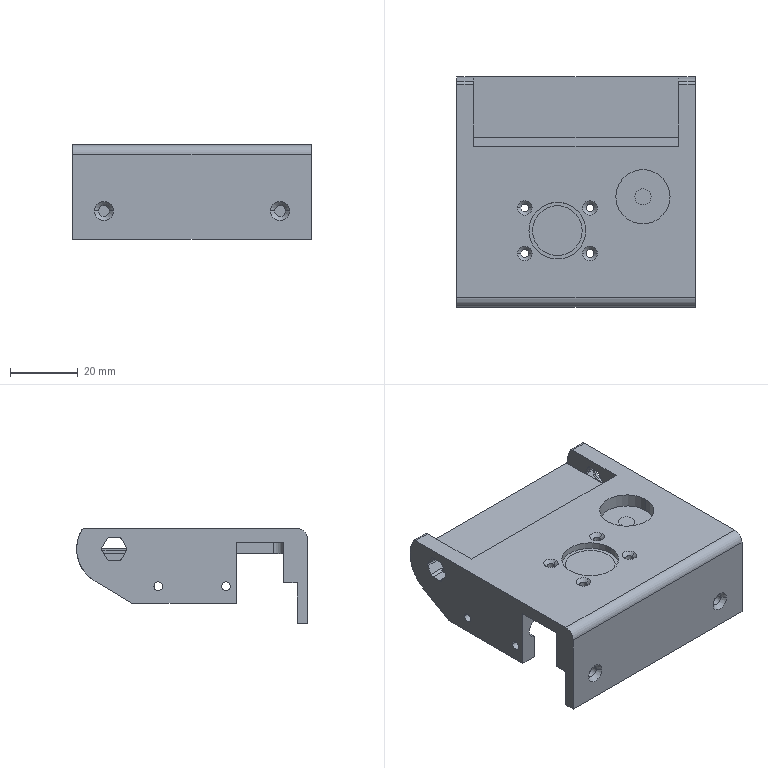NC program | NX | posted with a generic post | part box 70.5 x 68.1 x 28 mm
Lines 4053 to 5120 of 7250:
(ZLEVEL_PROFILE_COPY_COPY_1_COPY_1_COPY_1 , TOOL : D6R0.5)
N8062 T05 M6
N8064 G54
N8066 G17 G0 G90 X55.649 Y-26.288 B0. C0. S9500 M3
N8068 G43 Z30. H5
N8070 Z-5.051
N8072 G94 G1 Z-6.051 F1000.
N8074 X55.011 Y-26.4
N8076 G3 X54.516 Y-26.991 R0.6
N8078 G1 X54.515 Y-38.509 F3000.
N8080 X54.56 Y-38.51 Z-6.077
N8082 X54.601 Z-6.102
N8084 X54.603 Y-35.25
N8086 Y-30.25
N8088 X54.602 Y-26.99
N8090 X54.646 Z-6.128
N8092 X54.688 Y-26.989 Z-6.153
N8094 X54.689 Y-30.25
N8096 Y-35.25
N8098 X54.687 Y-38.511
N8100 X54.732 Z-6.179
N8102 X54.773 Y-38.512 Z-6.204
N8104 X54.775 Y-35.25
N8106 Y-30.25
N8108 X54.774 Y-26.989
N8110 X54.818 Y-26.988 Z-6.23
N8112 X54.86 Z-6.255
N8114 X54.861 Y-30.25
N8116 Y-35.25
N8118 X54.859 Y-38.512
N8120 X54.904 Y-38.513 Z-6.281
N8122 X54.945 Z-6.306
N8124 X54.947 Y-35.25
N8126 Y-30.25
N8128 X54.946 Y-26.987
N8130 X54.99 Z-6.332
N8132 X55.032 Y-26.986 Z-6.357
N8134 X55.033 Y-30.25
N8136 Y-35.25
N8138 X55.031 Y-38.514
N8140 X55.076 Z-6.383
N8142 X55.117 Y-38.515 Z-6.408
N8144 X55.119 Y-35.25
N8146 Y-30.25
N8148 X55.118 Y-26.986
N8150 X55.162 Y-26.985 Z-6.434
N8152 X55.204 Z-6.459
N8154 X55.205 Y-30.25
N8156 Y-35.25
N8158 X55.203 Y-38.515
N8160 X55.248 Y-38.516 Z-6.485
N8162 X55.289 Z-6.511
N8164 X55.29 Y-35.25
N8166 Y-30.25
N8168 Y-26.984
N8170 X55.333 Z-6.536
N8172 X55.376 Y-26.983 Z-6.562
N8174 Y-30.25
N8176 Y-35.25
N8178 X55.375 Y-38.517
N8180 X55.419 Z-6.587
N8182 X55.461 Y-38.518 Z-6.613
N8184 X55.462 Y-35.25
N8186 Y-30.25
N8188 Y-26.983
N8190 X55.505 Y-26.982 Z-6.638
N8192 X55.548 Z-6.664
N8194 Y-30.25
N8196 Y-35.25
N8198 X55.547 Y-38.518
N8200 X55.591 Y-38.519 Z-6.689
N8202 X55.633 Z-6.715
N8204 X55.634 Y-35.25
N8206 Y-30.25
N8208 Y-26.981
N8210 X55.677 Z-6.74
N8212 X55.72 Y-26.98 Z-6.766
N8214 Y-30.25
N8216 Y-35.25
N8218 X55.719 Y-38.52
N8220 X55.763 Z-6.791
N8222 X55.805 Y-38.521 Z-6.817
N8224 X55.806 Y-35.25
N8226 Y-30.25
N8228 Y-26.98
N8230 X55.849 Y-26.979 Z-6.842
N8232 X55.892 Z-6.868
N8234 Y-30.25
N8236 Y-35.25
N8238 X55.891 Y-38.521
N8240 X55.935 Y-38.522 Z-6.893
N8242 X55.977 Z-6.919
N8244 X55.978 Y-35.25
N8246 Y-30.25
N8248 Y-26.978
N8250 X56.021 Z-6.944
N8252 X56.064 Y-26.977 Z-6.97
N8254 Y-30.25
N8256 Y-35.25
N8258 X56.063 Y-38.523
N8260 X56.107 Z-6.995
N8262 X56.149 Z-7.021
N8264 X56.15 Y-35.25
N8266 Y-30.25
N8268 Y-26.977
N8270 X56.193 Z-7.047
N8272 X56.236 Y-26.976 Z-7.072
N8274 Y-30.25
N8276 Y-35.25
N8278 X56.235 Y-38.524
N8280 X56.279 Z-7.098
N8282 X56.321 Y-38.525 Z-7.123
N8284 X56.322 Y-35.25
N8286 Y-30.25
N8288 Y-26.976
N8290 X56.365 Y-26.975 Z-7.149
N8292 X56.408 Z-7.174
N8294 Y-30.25
N8296 Y-35.25
N8298 X56.407 Y-38.525
N8300 X56.451 Y-38.526 Z-7.2
N8302 X56.493 Z-7.225
N8304 X56.494 Y-35.25
N8306 Y-30.25
N8308 Y-26.974
N8310 X56.537 Z-7.251
N8312 X56.58 Z-7.276
N8314 Y-30.25
N8316 Y-35.25
N8318 X56.579 Y-38.527
N8320 X56.623 Z-7.302
N8322 X56.665 Z-7.327
N8324 X56.666 Y-35.25
N8326 Y-30.25
N8328 Y-26.973
N8330 X56.709 Z-7.353
N8332 X56.752 Y-26.972 Z-7.378
N8334 Y-30.25
N8336 Y-35.25
N8338 X56.751 Y-38.528
N8340 X56.795 Z-7.404
N8342 X56.837 Z-7.429
N8344 X56.838 Y-35.25
N8346 Y-30.25
N8348 Y-26.972
N8350 X56.881 Y-26.971 Z-7.455
N8352 X56.924 Z-7.48
N8354 Y-30.25
N8356 Y-35.25
N8358 X56.923 Y-38.529
N8360 X56.967 Z-7.506
N8362 X57.009 Y-38.53 Z-7.532
N8364 X57.01 Y-35.25
N8366 Y-30.25
N8368 Y-26.971
N8370 X57.053 Y-26.97 Z-7.557
N8372 X57.096 Z-7.583
N8374 Y-30.25
N8376 Y-35.25
N8378 X57.095 Y-38.53
N8380 X57.139 Y-38.531 Z-7.608
N8382 X57.181 Z-7.634
N8384 X57.182 Y-35.25
N8386 Y-30.25
N8388 Y-26.969
N8390 X57.225 Z-7.659
N8392 X57.268 Z-7.685
N8394 Y-30.25
N8396 Y-35.25
N8398 X57.267 Y-38.532
N8400 X57.311 Z-7.71
N8402 X57.353 Z-7.736
N8404 X57.354 Y-35.25
N8406 Y-30.25
N8408 Y-26.968
N8410 X57.397 Z-7.761
N8412 X57.44 Z-7.787
N8414 Y-30.25
N8416 Y-35.25
N8418 X57.439 Y-38.533
N8420 X57.483 Z-7.812
N8422 X57.525 Z-7.838
N8424 X57.526 Y-35.25
N8426 Y-30.25
N8428 Y-26.967
N8430 X57.569 Z-7.863
N8432 X57.612 Y-26.966 Z-7.889
N8434 Y-30.25
N8436 Y-35.25
N8438 X57.611 Y-38.534
N8440 X57.655 Z-7.914
N8442 X57.697 Z-7.94
N8444 X57.698 Y-35.25
N8446 Y-30.25
N8448 Y-26.966
N8450 X57.741 Z-7.965
N8452 X57.784 Y-26.965 Z-7.991
N8454 Y-30.25
N8456 Y-35.25
N8458 X57.783 Y-38.535
N8460 X57.827 Z-8.016
N8462 X57.869 Z-8.042
N8464 X57.87 Y-35.25
N8466 Y-30.25
N8468 Y-26.965
N8470 X57.913 Z-8.068
N8472 X57.956 Z-8.093
N8474 Y-30.25
N8476 Y-35.25
N8478 X57.955 Y-38.536
N8480 X57.999 Z-8.119
N8482 X58.041 Z-8.144
N8484 X58.042 Y-35.25
N8486 Y-30.25
N8488 Y-26.964
N8490 X58.085 Z-8.17
N8492 X58.128 Z-8.195
N8494 Y-30.25
N8496 Y-35.25
N8498 X58.127 Y-38.536
N8500 X58.171 Y-38.537 Z-8.221
N8502 X58.213 Z-8.246
N8504 X58.214 Y-35.25
N8506 Y-30.25
N8508 Y-26.964
N8510 X58.257 Y-26.963 Z-8.272
N8512 X58.3 Z-8.297
N8514 Y-30.25
N8516 Y-35.25
N8518 X58.299 Y-38.537
N8520 X58.343 Z-8.323
N8522 X58.385 Y-38.538 Z-8.348
N8524 X58.386 Y-35.25
N8526 Y-30.25
N8528 Y-26.963
N8530 X58.429 Z-8.374
N8532 X58.472 Y-26.962 Z-8.399
N8534 Y-30.25
N8536 Y-35.25
N8538 X58.471 Y-38.538
N8540 X58.515 Z-8.425
N8542 X58.557 Z-8.45
N8544 X58.558 Y-35.25
N8546 Y-30.25
N8548 Y-26.962
N8550 X58.601 Z-8.476
N8552 X58.644 Z-8.501
N8554 Y-30.25
N8556 Y-35.25
N8558 X58.643 Y-38.539
N8560 X58.687 Z-8.527
N8562 X58.729 Z-8.553
N8564 X58.73 Y-35.25
N8566 Y-30.25
N8568 Y-26.961
N8570 X58.773 Z-8.578
N8572 X58.816 Z-8.604
N8574 Y-30.25
N8576 Y-35.25
N8578 X58.815 Y-38.54
N8580 X58.859 Z-8.629
N8582 X58.901 Z-8.655
N8584 X58.902 Y-35.25
N8586 Y-30.25
N8588 Y-26.961
N8590 X58.945 Y-26.96 Z-8.68
N8592 X58.988 Z-8.706
N8594 Y-30.25
N8596 Y-35.25
N8598 X58.987 Y-38.54
N8600 X59.031 Y-38.541 Z-8.731
N8602 X59.073 Z-8.757
N8604 X59.074 Y-35.25
N8606 Y-30.25
N8608 Y-26.96
N8610 X59.117 Z-8.782
N8612 X59.16 Z-8.808
N8614 Y-30.25
N8616 Y-35.25
N8618 X59.159 Y-38.541
N8620 X59.203 Z-8.833
N8622 X59.245 Z-8.859
N8624 X59.246 Y-35.25
N8626 Y-30.25
N8628 X59.245 Y-26.959
N8630 X59.289 Z-8.884
N8632 X59.331 Z-8.91
N8634 X59.332 Y-30.25
N8636 Y-35.25
N8638 X59.331 Y-38.542
N8640 X59.375 Z-8.935
N8642 X59.417 Z-8.961
N8644 X59.418 Y-35.25
N8646 Y-30.25
N8648 X59.417 Y-26.959
N8650 X59.461 Z-8.986
N8652 X59.503 Z-9.012
N8654 X59.504 Y-30.25
N8656 Y-35.25
N8658 X59.503 Y-38.542
N8660 X59.547 Z-9.038
N8662 X59.589 Y-38.543 Z-9.063
N8664 X59.59 Y-35.25
N8666 Y-30.25
N8668 X59.589 Y-26.958
N8670 X59.633 Z-9.089
N8672 X59.675 Z-9.114
N8674 X59.676 Y-30.25
N8676 Y-35.25
N8678 X59.675 Y-38.543
N8680 X59.719 Z-9.14
N8682 X59.761 Z-9.165
N8684 X59.762 Y-35.25
N8686 Y-30.25
N8688 X59.761 Y-26.958
N8690 X59.805 Z-9.191
N8692 X59.847 Z-9.216
N8694 X59.848 Y-30.25
N8696 Y-35.25
N8698 X59.847 Y-38.543
N8700 X59.891 Z-9.242
N8702 X59.933 Z-9.267
N8704 X59.934 Y-35.25
N8706 Y-30.25
N8708 X59.933 Y-26.958
N8710 X59.977 Z-9.293
N8712 X60.019 Z-9.318
N8714 X60.02 Y-30.25
N8716 Y-35.25
N8718 X60.019 Y-38.544
N8720 X60.063 Z-9.344
N8722 X60.105 Z-9.369
N8724 X60.106 Y-35.25
N8726 Y-30.25
N8728 X60.105 Y-26.957
N8730 X60.149 Z-9.395
N8732 X60.191 Z-9.42
N8734 X60.192 Y-30.25
N8736 Y-35.25
N8738 X60.191 Y-38.544
N8740 X60.235 Z-9.446
N8742 X60.277 Z-9.471
N8744 X60.278 Y-35.25
N8746 Y-30.25
N8748 X60.277 Y-26.957
N8750 X60.321 Z-9.497
N8752 X60.363 Z-9.522
N8754 X60.364 Y-30.25
N8756 Y-35.25
N8758 X60.363 Y-38.544
N8760 X60.407 Y-38.545 Z-9.548
N8762 X60.449 Z-9.574
N8764 X60.45 Y-35.25
N8766 Y-30.25
N8768 X60.449 Y-26.957
N8770 X60.493 Z-9.599
N8772 X60.535 Z-9.625
N8774 X60.536 Y-30.25
N8776 Y-35.25
N8778 X60.535 Y-38.545
N8780 X60.579 Z-9.65
N8782 X60.621 Z-9.676
N8784 X60.622 Y-35.25
N8786 Y-30.25
N8788 X60.621 Y-26.956
N8790 X60.665 Z-9.701
N8792 X60.707 Z-9.727
N8794 X60.708 Y-30.25
N8796 Y-35.25
N8798 X60.707 Y-38.545
N8800 X60.751 Y-38.546 Z-9.752
N8802 X60.793 Z-9.778
N8804 X60.794 Y-35.25
N8806 Y-30.25
N8808 X60.793 Y-26.956
N8810 X60.837 Z-9.803
N8812 X60.879 Z-9.829
N8814 X60.88 Y-30.25
N8816 Y-35.25
N8818 X60.879 Y-38.546
N8820 X60.923 Z-9.854
N8822 X60.965 Z-9.88
N8824 X60.966 Y-35.25
N8826 Y-30.25
N8828 X60.965 Y-26.956
N8830 X61.009 Z-9.905
N8832 X61.051 Z-9.931
N8834 X61.052 Y-30.25
N8836 Y-35.25
N8838 X61.051 Y-38.546
N8840 X61.095 Z-9.956
N8842 X61.137 Z-9.982
N8844 X61.138 Y-35.25
N8846 Y-30.25
N8848 X61.137 Y-26.956
N8850 X61.181 Z-10.007
N8852 X61.223 Z-10.033
N8854 X61.224 Y-30.25
N8856 Y-35.25
N8858 X61.223 Y-38.546
N8860 X61.267 Z-10.059
N8862 X61.309 Z-10.084
N8864 X61.31 Y-35.25
N8866 Y-30.25
N8868 X61.309 Y-26.956
N8870 X61.353 Z-10.11
N8872 X61.395 Z-10.135
N8874 X61.396 Y-30.25
N8876 Y-35.25
N8878 X61.395 Y-38.547
N8880 X61.439 Z-10.161
N8882 X61.481 Z-10.186
N8884 X61.482 Y-35.25
N8886 Y-30.25
N8888 X61.481 Y-26.956
N8890 X61.525 Z-10.212
N8892 X61.567 Z-10.237
N8894 X61.568 Y-30.25
N8896 Y-35.25
N8898 X61.567 Y-38.547
N8900 X61.611 Z-10.263
N8902 X61.653 Z-10.288
N8904 X61.654 Y-35.25
N8906 Y-30.25
N8908 X61.653 Y-26.956
N8910 X61.697 Z-10.314
N8912 X61.739 Z-10.339
N8914 X61.74 Y-30.25
N8916 Y-35.25
N8918 X61.739 Y-38.547
N8920 X61.782 Z-10.365
N8922 X61.825 Z-10.39
N8924 X61.826 Y-35.25
N8926 Y-30.25
N8928 X61.825 Y-26.956
N8930 X61.869 Z-10.416
N8932 X61.911 Z-10.441
N8934 X61.912 Y-30.25
N8936 Y-35.25
N8938 X61.911 Y-38.547
N8940 X61.954 Z-10.467
N8942 X61.997 Z-10.492
N8944 X61.998 Y-35.25
N8946 Y-30.25
N8948 X61.997 Y-26.956
N8950 X62.041 Z-10.518
N8952 X62.083 Z-10.543
N8954 X62.084 Y-30.25
N8956 Y-35.25
N8958 X62.083 Y-38.548
N8960 X62.126 Z-10.569
N8962 X62.169 Z-10.595
N8964 Y-35.25
N8966 Y-30.25
N8968 Y-26.956
N8970 X62.212 Z-10.62
N8972 X62.255 Z-10.646
N8974 Y-30.25
N8976 Y-35.25
N8978 Y-38.548
N8980 X62.298 Z-10.671
N8982 X62.34 Z-10.697
N8984 X62.341 Y-35.25
N8986 Y-30.25
N8988 Y-26.956
N8990 X62.384 Z-10.722
N8992 X62.427 Z-10.748
N8994 Y-30.25
N8996 Y-35.25
N8998 X62.426 Y-38.548
N9000 X62.47 Z-10.773
N9002 X62.512 Z-10.799
N9004 X62.513 Y-35.25
N9006 Y-30.25
N9008 Y-26.956
N9010 X62.556 Z-10.824
N9012 X62.599 Z-10.85
N9014 X62.598 Y-30.007
N9016 X62.599 Y-30.25
N9018 Y-35.25
N9020 X62.598 Y-38.275
N9022 Y-38.548
N9024 X62.642 Z-10.875
N9026 X62.684 Z-10.901
N9028 X62.682 Y-37.931
N9030 X62.685 Y-35.25
N9032 Y-30.25
N9034 X62.684 Y-30.007
N9036 X62.685 Y-26.956
N9038 X62.728 Z-10.926
N9040 X62.771 Y-26.957 Z-10.952
N9042 X62.769 Y-30.007
N9044 X62.771 Y-30.25
N9046 Y-35.25
N9048 X62.768 Y-37.931
N9050 X62.77 Y-38.548
N9052 X62.814 Z-10.977
N9054 X62.856 Z-11.003
N9056 X62.853 Y-37.931
N9058 X62.857 Y-35.25
N9060 Y-30.25
N9062 X62.855 Y-30.007
N9064 X62.857 Y-26.957
N9066 X62.9 Z-11.028
N9068 X62.943 Z-11.054
N9070 X62.939 Y-29.663
N9072 X62.943 Y-30.25
N9074 Y-35.25
N9076 X62.941 Y-38.275
N9078 X62.942 Y-38.548
N9080 X62.986 Z-11.08
N9082 X63.028 Z-11.105
N9084 X63.025 Y-37.931
N9086 X63.029 Y-35.25
N9088 Y-30.25
N9090 X63.025 Y-29.663
N9092 X63.029 Y-26.957
N9094 X63.072 Z-11.131
N9096 X63.115 Z-11.156
N9098 X63.111 Y-29.663
N9100 X63.115 Y-30.25
N9102 Y-35.25
N9104 X63.111 Y-37.931
N9106 X63.114 Y-38.548
N9108 X63.158 Z-11.182
N9110 X63.2 Z-11.207
N9112 X63.197 Y-37.931
N9114 X63.201 Y-35.25
N9116 Y-30.25
N9118 X63.196 Y-29.663
N9120 X63.201 Y-26.957
N9122 X63.244 Z-11.233
N9124 X63.287 Z-11.258
N9126 X63.282 Y-29.663
N9128 X63.287 Y-30.25
N9130 Y-35.25
N9132 X63.285 Y-38.549
N9134 X63.33 Z-11.284
N9136 X63.371 Z-11.309
N9138 X63.373 Y-35.25
N9140 Y-30.25
N9142 X63.368 Y-29.663
N9144 X63.373 Y-26.957
N9146 X63.416 Z-11.335
N9148 X63.459 Y-26.958 Z-11.36
N9150 X63.454 Y-29.663
N9152 X63.459 Y-30.25
N9154 Y-35.25
N9156 X63.457 Y-38.549
N9158 X63.501 Z-11.386
N9160 X63.543 Z-11.411
N9162 X63.545 Y-35.25
N9164 Y-30.25
N9166 X63.539 Y-29.663
N9168 X63.545 Y-26.958
N9170 X63.588 Z-11.437
N9172 X63.63 Z-11.462
N9174 X63.625 Y-29.663
N9176 X63.631 Y-30.25
N9178 Y-35.25
N9180 X63.629 Y-38.549
N9182 X63.673 Z-11.488
N9184 X63.715 Z-11.513
N9186 X63.716 Y-35.519
N9188 X63.717 Y-35.25
N9190 Y-30.25
N9192 X63.711 Y-29.663
N9194 X63.716 Y-26.958
N9196 X63.76 Z-11.539
N9198 X63.802 Z-11.564
N9200 X63.797 Y-29.663
N9202 X63.803 Y-30.25
N9204 Y-35.25
N9206 X63.8 Y-35.864
N9208 X63.801 Y-38.549
N9210 X63.845 Z-11.59
N9212 X63.887 Z-11.616
N9214 X63.885 Y-35.864
N9216 X63.889 Y-35.25
N9218 Y-30.25
N9220 X63.883 Y-29.663
N9222 X63.888 Y-26.958
N9224 X63.932 Y-26.959 Z-11.641
N9226 X63.974 Z-11.667
N9228 X63.971 Y-30.007
N9230 X63.975 Y-30.25
N9232 Y-35.25
N9234 X63.972 Y-38.549
N9236 X64.016 Z-11.692
N9238 X64.057 Z-11.718
N9240 X64.061 Y-35.25
N9242 Y-30.25
N9244 X64.051 Y-29.663
N9246 X64.059 Y-26.959
N9248 X64.102 Z-11.743
N9250 X64.144 Z-11.769
N9252 X64.135 Y-29.663
N9254 X64.147 Y-30.25
N9256 Y-35.25
N9258 X64.142 Y-38.549
N9260 X64.186 Z-11.794
N9262 X64.227 Z-11.82
N9264 X64.223 Y-38.275
N9266 X64.233 Y-35.25
N9268 Y-30.25
N9270 X64.219 Y-29.663
N9272 X64.23 Y-26.96
N9274 X64.273 Z-11.845
N9276 X64.315 Z-11.871
N9278 X64.303 Y-29.663
N9280 X64.319 Y-30.25
N9282 Y-35.25
N9284 X64.301 Y-37.931
N9286 X64.312 Y-38.549
N9288 X64.356 Z-11.896
N9290 X64.397 Z-11.922
N9292 X64.385 Y-37.931
N9294 X64.405 Y-35.25
N9296 Y-30.25
N9298 X64.387 Y-29.663
N9300 X64.401 Y-26.96
N9302 X64.444 Z-11.947
N9304 X64.486 Y-26.961 Z-11.973
N9306 X64.482 Y-30.007
N9308 X64.491 Y-30.25
N9310 Y-35.25
N9312 X64.469 Y-37.931
N9314 X64.482 Y-38.549
N9316 X64.527 Z-11.998
N9318 X64.567 Z-12.024
N9320 G2 X64.577 Y-35.25 R56.425
N9322 G1 Y-30.25
N9324 X64.554 Y-29.663
N9326 X64.572 Y-26.961
N9328 X64.615 Z-12.049
N9330 X64.657 Z-12.075
N9332 X64.639 Y-29.663
N9334 X64.663 Y-30.25
N9336 Y-35.25
N9338 G3 X64.653 Y-38.549 R51.896
N9340 G1 X64.697 Z-12.101
N9342 X64.738 Z-12.126
N9344 G2 X64.749 Y-35.25 R48.139
N9346 G1 Y-30.25
N9348 X64.724 Y-29.663
N9350 X64.742 Y-26.962
N9352 X64.786 Z-12.152
N9354 X64.828 Z-12.177
N9356 X64.809 Y-29.663
N9358 X64.835 Y-30.25
N9360 Y-35.25
N9362 G3 X64.823 Y-38.549 R44.89
N9364 G1 X64.868 Y-38.55 Z-12.203
N9366 X64.908 Z-12.228
N9368 G2 X64.921 Y-35.25 R42.052
N9370 G1 Y-30.25
N9372 X64.894 Y-29.663
N9374 X64.913 Y-26.962
N9376 X64.957 Z-12.254
N9378 X64.999 Y-26.963 Z-12.279
N9380 X64.996 Y-27.251
N9382 X64.98 Y-29.663
N9384 X65.007 Y-30.25
N9386 Y-35.25
N9388 G3 X64.993 Y-38.55 R39.225
N9390 G1 X65.038 Z-12.305
N9392 X65.078 Z-12.33
N9394 G2 X65.093 Y-35.25 R37.273
N9396 G1 Y-30.25
N9398 G2 X65.084 Y-26.963 R41.614
N9400 G1 X65.128 Z-12.356
N9402 X65.169 Z-12.381
N9404 G3 X65.179 Y-30.25 R39.32
N9406 G1 Y-35.25
N9408 G3 X65.164 Y-38.55 R35.506
N9410 G1 X65.208 Z-12.407
N9412 X65.249 Z-12.432
N9414 G2 X65.265 Y-35.25 R33.187
N9416 G1 Y-30.25
N9418 G2 X65.255 Y-26.964 R37.265
N9420 G1 X65.299 Z-12.458
N9422 X65.337 Z-12.483
N9424 G3 X65.351 Y-30.25 R34.656
N9426 G1 Y-35.25
N9428 G3 X65.331 Y-38.55 R31.308
N9430 G1 X65.379 Z-12.509
N9432 X65.412 Z-12.534
N9434 G2 X65.437 Y-35.25 R29.3
N9436 G1 Y-30.25
N9438 G2 X65.418 Y-26.965 R31.712
N9440 G1 X65.466 Z-12.56
N9442 X65.5 Z-12.586
N9444 G3 X65.523 Y-30.25 R29.549
N9446 G1 Y-35.25
N9448 G3 X65.493 Y-38.55 R27.132
N9450 G1 X65.54 Z-12.612
N9452 X65.576 Z-12.638
N9454 G2 X65.608 Y-35.25 R25.738
N9456 G1 Y-30.25
N9458 G2 X65.582 Y-26.966 R28.254
N9460 G1 X65.626 Z-12.665
N9462 X65.664 Z-12.691
N9464 G3 X65.692 Y-30.25 R27.78
N9466 G1 Y-35.25
N9468 G3 X65.658 Y-38.55 R24.917
N9470 G1 X65.701 Z-12.718
N9472 X65.739 Z-12.744
N9474 G2 X65.776 Y-35.25 R23.927
N9476 G1 Y-30.25
N9478 G2 X65.745 Y-26.967 R26.908
N9480 G1 X65.788 Z-12.772
N9482 X65.828 Z-12.799
N9484 G3 X65.859 Y-30.25 R27.201
N9486 G1 Y-35.25
N9488 G3 X65.821 Y-38.55 R23.227
N9490 G1 X65.865 Z-12.826
N9492 X65.905 Z-12.853
N9494 G2 X65.942 Y-35.25 R22.927
N9496 G1 Y-30.25
N9498 G2 X65.911 Y-26.968 R27.436
N9500 G1 X65.955 Z-12.881
N9502 X65.994 Y-26.969 Z-12.909
N9504 G3 X66.024 Y-30.25 R28.371
N9506 G1 Y-35.25
N9508 G3 X65.988 Y-38.55 R23.27
N9510 G1 X66.034 Z-12.937
N9512 X66.069 Z-12.965
N9514 G2 X66.106 Y-35.25 R22.839
N9516 G1 Y-30.25
N9518 G2 X66.077 Y-26.97 R28.653
N9520 G1 X66.126 Z-12.993
N9522 X66.161 Z-13.022
N9524 G3 X66.188 Y-30.25 R28.753
N9526 G1 Y-35.25
N9528 G3 X66.151 Y-38.55 R22.238
N9530 G1 X66.203 Z-13.051
N9532 X66.234 Z-13.08
N9534 G2 X66.269 Y-35.25 R22.107
N9536 G1 Y-30.25
N9538 G2 X66.245 Y-26.971 R30.224
N9540 G1 X66.292 Y-26.972 Z-13.109
N9542 X66.329 Z-13.138
N9544 G3 X66.349 Y-30.25 R34.224
N9546 G1 Y-35.25
N9548 G3 X66.318 Y-38.55 R22.502
N9550 G1 X66.358 Z-13.167
N9552 X66.394 Z-13.197
N9554 G2 X66.429 Y-35.25 R22.154
N9556 G1 Y-30.25
N9558 G2 X66.409 Y-26.973 R35.085
N9560 G1 X66.451 Y-26.974 Z-13.227
N9562 X66.489 Y-26.975 Z-13.257
N9564 G3 X66.509 Y-30.25 R37.644
N9566 G1 Y-35.25
N9568 G3 X66.471 Y-38.55 R21.406
N9570 G1 X66.513 Z-13.287
N9572 X66.549 Z-13.317
N9574 G2 X66.587 Y-35.25 R21.087
N9576 G1 Y-30.25
N9578 G2 X66.57 Y-26.976 R41.79
N9580 G1 X66.613 Y-26.977 Z-13.348
N9582 X66.653 Z-13.378
N9584 G3 X66.666 Y-30.25 R48.238
N9586 G1 Y-35.25
N9588 G3 X66.628 Y-38.55 R21.161
N9590 G1 X66.671 Z-13.409
N9592 X66.707 Z-13.44
N9594 X66.673 Y-37.242
N9596 G2 X66.744 Y-35.25 R13.926
N9598 G1 Y-30.373
N9600 G2 X66.73 Y-26.979 R61.087
N9602 G1 X66.774 Y-26.981 Z-13.471
N9604 X66.807 Z-13.501
N9606 G3 X66.82 Y-30.547 R76.412
N9608 G1 Y-35.25
N9610 G3 X66.785 Y-38.55 R21.514
N9612 G1 X66.83 Z-13.532
N9614 X66.863 Z-13.563
N9616 G2 X66.896 Y-35.25 R21.959
N9618 G1 Y-30.695
N9620 G2 X66.885 Y-26.983 R98.077
N9622 G1 X66.927 Y-26.985 Z-13.594
N9624 X66.963 Z-13.625
N9626 G3 X66.97 Y-30.823 R130.255
N9628 G1 Y-35.25
N9630 G3 X66.941 Y-38.55 R22.834
N9632 G1 X66.983 Z-13.656
N9634 X67.017 Z-13.687
N9636 X67.012 Y-38.275
N9638 X66.981 Y-37.124
N9640 G2 X67.043 Y-35.25 R15.91
N9642 G1 Y-30.936
N9644 G2 X67.039 Y-26.988 R184.318
N9646 G1 X67.08 Y-26.989 Z-13.718
N9648 X67.115 Y-26.99 Z-13.749
N9650 X67.107 Y-27.596
N9652 X67.115 Y-31.04
N9654 Y-35.25
N9656 G3 X67.054 Y-37.242 R15.668
N9658 G1 X67.085 Y-38.55
N9660 X67.121 Z-13.78
N9662 X67.153 Z-13.811
N9664 X67.122 Y-37.242
N9666 G2 X67.186 Y-35.25 R15.004
N9668 G1 Y-31.135
N9670 X67.183 Y-27.596
N9672 X67.191 Y-26.992
N9674 X67.234 Y-26.993 Z-13.843
N9676 X67.267 Y-26.994 Z-13.874
N9678 X67.255 Y-31.221
N9680 Y-35.25
N9682 G3 X67.19 Y-37.242 R14.676
N9684 G1 X67.221 Y-38.55
N9686 X67.257 Z-13.905
N9688 X67.289 Z-13.936
N9690 X67.258 Y-37.242
N9692 G2 X67.324 Y-35.25 R14.681
N9694 G1 Y-31.306
N9696 X67.342 Y-26.997
N9698 X67.379 Y-26.999 Z-13.967
N9700 X67.407 Y-27. Z-13.999
N9702 X67.392 Y-31.38
N9704 Y-35.25
N9706 G3 X67.327 Y-37.242 R14.909
N9708 G1 X67.358 Y-38.55
N9710 X67.395 Z-14.031
N9712 X67.427 Z-14.063
N9714 X67.396 Y-37.242
N9716 G2 X67.461 Y-35.25 R14.792
N9718 G1 Y-31.456
N9720 X67.473 Y-27.004
N9722 X67.515 Y-27.007 Z-14.095
N9724 X67.539 Y-27.008 Z-14.128
N9726 X67.529 Y-31.525
N9728 Y-35.25
N9730 G3 X67.466 Y-37.242 R14.969
N9732 G1 X67.497 Y-38.55
N9734 X67.538 Z-14.161
N9736 X67.569 Z-14.195
N9738 X67.537 Y-37.242
N9740 G2 X67.598 Y-35.25 R15.483
N9742 G1 Y-31.592
N9744 X67.594 Y-31.041
N9746 X67.608 Y-27.012
N9748 X67.648 Y-27.014 Z-14.229
N9750 X67.677 Y-27.016 Z-14.263
N9752 X67.665 Y-31.385
N9754 X67.667 Y-31.659
N9756 Y-35.25
N9758 G3 X67.609 Y-37.242 R16.42
N9760 G1 X67.642 Y-38.55
N9762 X67.68 Z-14.297
N9764 X67.712 Z-14.332
N9766 X67.708 Y-38.275
N9768 X67.68 Y-37.105
N9770 G2 X67.736 Y-35.25 R17.399
N9772 G1 Y-31.719
N9774 X67.733 Y-31.385
N9776 X67.742 Y-27.024
N9778 X67.778 Y-27.03 Z-14.366
N9780 X67.807 Y-27.034 Z-14.401
N9782 X67.805 Y-31.779
N9784 Y-35.25
N9786 G3 X67.749 Y-37.242 R16.775
N9788 G1 X67.777 Y-38.55
N9790 X67.812 Z-14.436
N9792 X67.842 Z-14.471
N9794 X67.807 Y-36.553
N9796 X67.808 Y-36.208
N9798 X67.873 Y-35.25
N9800 Y-31.834
N9802 X67.864 Y-31.041
N9804 X67.872 Y-27.043
N9806 X67.909 Y-27.049 Z-14.507
N9808 X67.938 Y-27.053 Z-14.542
N9810 X67.939 Y-27.251
N9812 X67.931 Y-31.041
N9814 X67.94 Y-31.886
N9816 Y-35.25
N9818 X67.874 Y-36.208
N9820 X67.873 Y-36.553
N9822 X67.908 Y-38.55
N9824 X67.943 Z-14.578
N9826 X67.974 Z-14.613
N9828 X67.939 Y-36.553
N9830 X67.94 Y-36.208
N9832 X68.006 Y-35.25
N9834 Y-31.939
N9836 X67.999 Y-31.041
N9838 X68.004 Y-27.063
N9840 X68.069 Y-27.09 Z-14.685
N9842 X68.071 Y-27.251
N9844 X68.064 Y-31.041
N9846 X68.072 Y-31.985
N9848 Y-35.25
N9850 X68.007 Y-36.208
N9852 X68.006 Y-36.553
N9854 X68.041 Y-38.55
N9856 X68.077 Z-14.721
N9858 X68.105 Z-14.757
N9860 X68.071 Y-36.553
N9862 X68.072 Y-36.208
N9864 X68.138 Y-35.25
N9866 Y-32.03
N9868 X68.132 Y-31.73
N9870 X68.134 Y-27.128
N9872 X68.199 Y-27.167 Z-14.83
N9874 X68.196 Y-31.73
N9876 X68.202 Y-32.075
N9878 Y-35.25
N9880 X68.136 Y-36.208
N9882 X68.135 Y-36.553
N9884 X68.17 Y-38.55
N9886 X68.212 Z-14.866
N9888 X68.236 Z-14.903
N9890 X68.2 Y-36.553
N9892 X68.201 Y-36.208
N9894 X68.266 Y-35.25
N9896 Y-32.114
N9898 X68.26 Y-31.73
N9900 X68.261 Y-27.596
N9902 X68.264 Y-27.205
N9904 X68.331 Y-27.244 Z-14.977
N9906 G3 X68.328 Y-32.074 R220.248
N9908 G1 X68.33 Y-32.153
N9910 Y-35.25
N9912 X68.266 Y-36.208
N9914 Y-36.553
N9916 X68.302 Y-38.55
N9918 X68.341 Z-15.014
N9920 X68.368 Z-15.052
N9922 X68.332 Y-36.553
N9924 Y-36.208
N9926 X68.393 Y-35.25
N9928 Y-32.189
N9930 G2 X68.391 Y-27.412 R392.445
N9932 G1 X68.425 Y-27.512 Z-15.089
N9934 X68.456 Y-27.611 Z-15.127
N9936 G3 X68.452 Y-32.074 R232.711
N9938 G1 X68.455 Y-32.224
N9940 Y-35.25
N9942 X68.397 Y-36.208
N9944 X68.396 Y-36.553
N9946 X68.429 Y-38.55
N9948 X68.461 Z-15.165
N9950 X68.489 Z-15.203
N9952 X68.456 Y-36.553
N9954 X68.457 Y-36.208
N9956 X68.518 Y-35.25
N9958 Y-32.256
N9960 X68.512 Y-32.074
N9962 G2 X68.519 Y-27.81 R224.95
N9964 G1 X68.552 Y-27.906 Z-15.242
N9966 X68.58 Y-28.002 Z-15.28
N9968 G3 X68.574 Y-32.074 R267.581
N9970 G1 X68.579 Y-32.287
N9972 Y-35.25
N9974 X68.517 Y-36.208
N9976 Y-36.553
N9978 X68.549 Y-38.55
N9980 X68.582 Z-15.318
N9982 X68.61 Z-15.357
N9984 X68.577 Y-36.553
N9986 X68.578 Y-36.208
N9988 X68.64 Y-35.25
N9990 Y-32.314
N9992 X68.635 Y-32.074
N9994 X68.636 Y-28.629
N9996 X68.639 Y-28.187
N9998 X68.672 Y-28.279 Z-15.396
N10000 X68.701 Y-28.372 Z-15.434
N10002 X68.697 Y-32.074
N10004 X68.7 Y-32.341
N10006 Y-35.25
N10008 X68.639 Y-36.208
N10010 X68.638 Y-36.553
N10012 X68.671 Y-38.55
N10014 X68.704 Z-15.473
N10016 X68.733 Z-15.513
N10018 X68.7 Y-36.553
N10020 Y-36.208
N10022 X68.759 Y-35.25
N10024 Y-32.365
N10026 X68.756 Y-32.074
N10028 X68.758 Y-28.533
N10030 X68.817 Y-28.658 Z-15.592
N10032 X68.813 Y-32.074
N10034 X68.819 Y-32.386
N10036 Y-35.25
N10038 X68.762 Y-36.208
N10040 G3 X68.794 Y-38.55 R73.624
N10042 G1 X68.829 Z-15.632
N10044 X68.857 Z-15.672
N10046 G2 X68.823 Y-36.208 R71.199
N10048 G1 X68.877 Y-35.25
N10050 Y-32.408
N10052 X68.868 Y-31.73
N10054 X68.869 Y-28.739
N10056 X68.925 Y-28.82 Z-15.753
N10058 X68.929 Y-32.074
N10060 X68.936 Y-32.426
N10062 Y-35.25
N10064 X68.884 Y-36.208
N10066 G3 X68.916 Y-38.55 R91.878
N10068 G1 X68.945 Z-15.793
N10070 X68.97 Z-15.834
N10072 G2 X68.939 Y-36.208 R81.312
N10074 G1 X68.993 Y-35.25
N10076 Y-32.441
N10078 X68.984 Y-28.902
N10080 X69.046 Y-28.98 Z-15.916
N10082 X69.05 Y-32.419
N10084 Y-32.457
N10086 Y-35.25
N10088 X68.994 Y-36.208
N10090 G3 X69.024 Y-38.55 R81.211
N10092 G1 X69.054 Z-15.957
N10094 X69.079 Z-15.998
N10096 G2 X69.048 Y-36.208 R81.203
N10098 G1 X69.107 Y-35.25
N10100 Y-32.469
N10102 X69.104 Y-32.419
N10104 X69.101 Y-29.008
N10106 X69.155 Y-29.023 Z-16.081
N10108 X69.158 Y-32.419
N10110 X69.162 Y-32.478
N10112 Y-35.25
N10114 X69.103 Y-36.208
N10116 G3 X69.134 Y-38.55 R80.063
N10118 G1 X69.164 Z-16.123
N10120 X69.189 Z-16.165
N10122 G2 X69.158 Y-36.208 R78.795
N10124 G1 X69.217 Y-35.25
N10126 Y-32.487
N10128 X69.212 Y-32.419
N10130 X69.209 Y-29.038
N10132 X69.263 Y-29.054 Z-16.249
N10134 X69.262 Y-29.318
N10136 X69.266 Y-32.419
N10138 X69.271 Y-32.493
N10140 Y-35.25
N10142 X69.212 Y-36.208
N10144 G3 X69.245 Y-38.55 R77.56
N10146 G1 X69.275 Z-16.291
N10148 X69.3 Z-16.333
N10150 G2 X69.268 Y-36.208 R76.356
N10152 G1 X69.325 Y-35.25
N10154 Y-32.496
N10156 X69.321 Y-32.419
N10158 X69.318 Y-29.069
N10160 X69.373 Y-29.085 Z-16.418
N10162 X69.375 Y-32.419
N10164 X69.378 Y-32.499
N10166 Y-35.25
N10168 X69.323 Y-36.208
N10170 G3 X69.357 Y-38.55 R75.183
N10172 G1 X69.386 Z-16.46
N10174 X69.413 Z-16.503
N10176 G2 X69.379 Y-36.208 R75.741
N10178 G1 X69.43 Y-35.25
N10180 Y-32.499
N10182 X69.428 Y-32.419
N10184 X69.425 Y-29.318
N10186 X69.429 Y-29.029
N10188 X69.458 Y-28.923 Z-16.546
N10190 X69.483 Y-28.818 Z-16.589